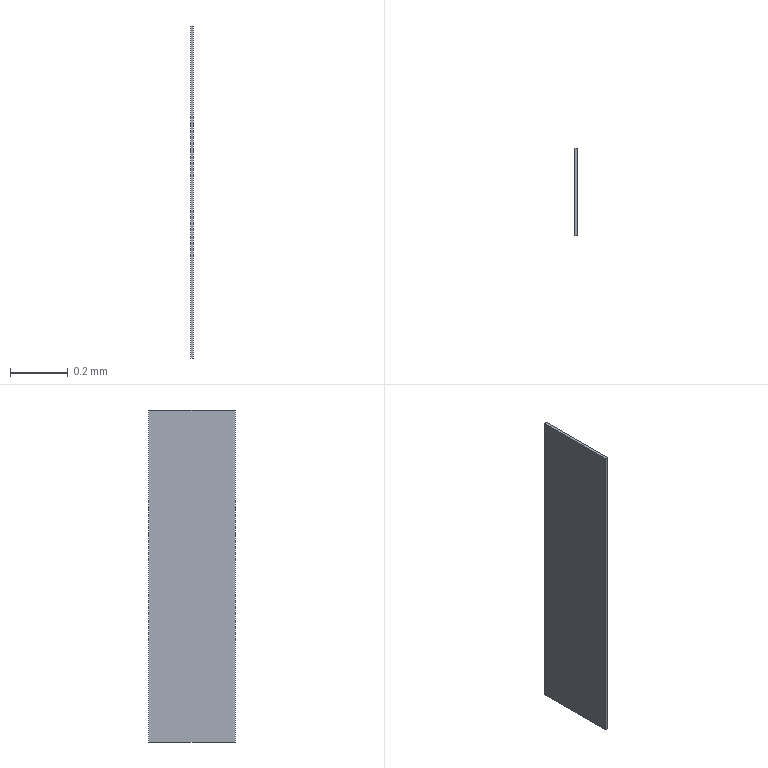Part | Creo | 1 solid | 6 faces | box 0.01 x 0.3 x 1.15 mm | volume 0.00345 mm3 | plane 6
STEP:
#1=CARTESIAN_POINT('',(0.,0.,0.));
#2=DIRECTION('',(0.,0.,1.));
#3=DIRECTION('',(1.,0.,0.));
#4=AXIS2_PLACEMENT_3D('',#1,#2,#3);
#5=CARTESIAN_POINT('',(0.12,-6.2,0.525));
#6=VERTEX_POINT('',#5);
#7=CARTESIAN_POINT('',(0.12,-6.2,1.675));
#8=VERTEX_POINT('',#7);
#9=CARTESIAN_POINT('',(0.12,-6.2,0.525));
#10=DIRECTION('',(0.,0.,1.));
#11=VECTOR('',#10,1.15);
#12=LINE('',#9,#11);
#13=EDGE_CURVE('',#6,#8,#12,.T.);
#14=ORIENTED_EDGE('',*,*,#13,.F.);
#15=CARTESIAN_POINT('',(0.12,-6.5,0.525));
#16=VERTEX_POINT('',#15);
#17=CARTESIAN_POINT('',(0.12,-6.5,0.525));
#18=DIRECTION('',(0.,1.,0.));
#19=VECTOR('',#18,0.3);
#20=LINE('',#17,#19);
#21=EDGE_CURVE('',#16,#6,#20,.T.);
#22=ORIENTED_EDGE('',*,*,#21,.F.);
#23=CARTESIAN_POINT('',(0.12,-6.5,1.675));
#24=VERTEX_POINT('',#23);
#25=CARTESIAN_POINT('',(0.12,-6.5,1.675));
#26=DIRECTION('',(0.,0.,-1.));
#27=VECTOR('',#26,1.15);
#28=LINE('',#25,#27);
#29=EDGE_CURVE('',#24,#16,#28,.T.);
#30=ORIENTED_EDGE('',*,*,#29,.F.);
#31=CARTESIAN_POINT('',(0.12,-6.2,1.675));
#32=DIRECTION('',(0.,-1.,0.));
#33=VECTOR('',#32,0.3);
#34=LINE('',#31,#33);
#35=EDGE_CURVE('',#8,#24,#34,.T.);
#36=ORIENTED_EDGE('',*,*,#35,.F.);
#37=EDGE_LOOP('',(#14,#22,#30,#36));
#38=FACE_OUTER_BOUND('',#37,.F.);
#39=CARTESIAN_POINT('',(0.12,0.,0.));
#40=DIRECTION('',(1.,0.,0.));
#41=DIRECTION('',(0.,-1.,0.));
#42=AXIS2_PLACEMENT_3D('',#39,#40,#41);
#43=PLANE('',#42);
#44=ADVANCED_FACE('',(#38),#43,.T.);
#45=CARTESIAN_POINT('',(0.11,-6.2,0.525));
#46=VERTEX_POINT('',#45);
#47=CARTESIAN_POINT('',(0.11,-6.2,1.675));
#48=VERTEX_POINT('',#47);
#49=CARTESIAN_POINT('',(0.11,-6.2,0.525));
#50=DIRECTION('',(0.,0.,1.));
#51=VECTOR('',#50,1.15);
#52=LINE('',#49,#51);
#53=EDGE_CURVE('',#46,#48,#52,.T.);
#54=ORIENTED_EDGE('',*,*,#53,.F.);
#55=CARTESIAN_POINT('',(0.11,-6.2,0.525));
#56=DIRECTION('',(1.,0.,0.));
#57=VECTOR('',#56,0.01);
#58=LINE('',#55,#57);
#59=EDGE_CURVE('',#46,#6,#58,.T.);
#60=ORIENTED_EDGE('',*,*,#59,.T.);
#61=ORIENTED_EDGE('',*,*,#13,.T.);
#62=CARTESIAN_POINT('',(0.11,-6.2,1.675));
#63=DIRECTION('',(1.,0.,0.));
#64=VECTOR('',#63,0.01);
#65=LINE('',#62,#64);
#66=EDGE_CURVE('',#48,#8,#65,.T.);
#67=ORIENTED_EDGE('',*,*,#66,.F.);
#68=EDGE_LOOP('',(#54,#60,#61,#67));
#69=FACE_OUTER_BOUND('',#68,.F.);
#70=CARTESIAN_POINT('',(0.,-6.2,0.525));
#71=DIRECTION('',(0.,1.,0.));
#72=DIRECTION('',(0.,0.,1.));
#73=AXIS2_PLACEMENT_3D('',#70,#71,#72);
#74=PLANE('',#73);
#75=ADVANCED_FACE('',(#69),#74,.T.);
#76=ORIENTED_EDGE('',*,*,#53,.T.);
#77=CARTESIAN_POINT('',(0.11,-6.5,1.675));
#78=VERTEX_POINT('',#77);
#79=CARTESIAN_POINT('',(0.11,-6.2,1.675));
#80=DIRECTION('',(0.,-1.,0.));
#81=VECTOR('',#80,0.3);
#82=LINE('',#79,#81);
#83=EDGE_CURVE('',#48,#78,#82,.T.);
#84=ORIENTED_EDGE('',*,*,#83,.T.);
#85=CARTESIAN_POINT('',(0.11,-6.5,0.525));
#86=VERTEX_POINT('',#85);
#87=CARTESIAN_POINT('',(0.11,-6.5,1.675));
#88=DIRECTION('',(0.,0.,-1.));
#89=VECTOR('',#88,1.15);
#90=LINE('',#87,#89);
#91=EDGE_CURVE('',#78,#86,#90,.T.);
#92=ORIENTED_EDGE('',*,*,#91,.T.);
#93=CARTESIAN_POINT('',(0.11,-6.5,0.525));
#94=DIRECTION('',(0.,1.,0.));
#95=VECTOR('',#94,0.3);
#96=LINE('',#93,#95);
#97=EDGE_CURVE('',#86,#46,#96,.T.);
#98=ORIENTED_EDGE('',*,*,#97,.T.);
#99=EDGE_LOOP('',(#76,#84,#92,#98));
#100=FACE_OUTER_BOUND('',#99,.F.);
#101=CARTESIAN_POINT('',(0.11,-11.395,4.186));
#102=DIRECTION('',(1.,0.,0.));
#103=DIRECTION('',(0.,1.,0.));
#104=AXIS2_PLACEMENT_3D('',#101,#102,#103);
#105=PLANE('',#104);
#106=ADVANCED_FACE('',(#100),#105,.F.);
#107=ORIENTED_EDGE('',*,*,#83,.F.);
#108=ORIENTED_EDGE('',*,*,#66,.T.);
#109=ORIENTED_EDGE('',*,*,#35,.T.);
#110=CARTESIAN_POINT('',(0.11,-6.5,1.675));
#111=DIRECTION('',(1.,0.,0.));
#112=VECTOR('',#111,0.01);
#113=LINE('',#110,#112);
#114=EDGE_CURVE('',#78,#24,#113,.T.);
#115=ORIENTED_EDGE('',*,*,#114,.F.);
#116=EDGE_LOOP('',(#107,#108,#109,#115));
#117=FACE_OUTER_BOUND('',#116,.F.);
#118=CARTESIAN_POINT('',(0.,-6.2,1.675));
#119=DIRECTION('',(0.,0.,1.));
#120=DIRECTION('',(0.,-1.,0.));
#121=AXIS2_PLACEMENT_3D('',#118,#119,#120);
#122=PLANE('',#121);
#123=ADVANCED_FACE('',(#117),#122,.T.);
#124=ORIENTED_EDGE('',*,*,#91,.F.);
#125=ORIENTED_EDGE('',*,*,#114,.T.);
#126=ORIENTED_EDGE('',*,*,#29,.T.);
#127=CARTESIAN_POINT('',(0.11,-6.5,0.525));
#128=DIRECTION('',(1.,0.,0.));
#129=VECTOR('',#128,0.01);
#130=LINE('',#127,#129);
#131=EDGE_CURVE('',#86,#16,#130,.T.);
#132=ORIENTED_EDGE('',*,*,#131,.F.);
#133=EDGE_LOOP('',(#124,#125,#126,#132));
#134=FACE_OUTER_BOUND('',#133,.F.);
#135=CARTESIAN_POINT('',(0.,-6.5,1.675));
#136=DIRECTION('',(0.,-1.,0.));
#137=DIRECTION('',(0.,0.,-1.));
#138=AXIS2_PLACEMENT_3D('',#135,#136,#137);
#139=PLANE('',#138);
#140=ADVANCED_FACE('',(#134),#139,.T.);
#141=ORIENTED_EDGE('',*,*,#97,.F.);
#142=ORIENTED_EDGE('',*,*,#131,.T.);
#143=ORIENTED_EDGE('',*,*,#21,.T.);
#144=ORIENTED_EDGE('',*,*,#59,.F.);
#145=EDGE_LOOP('',(#141,#142,#143,#144));
#146=FACE_OUTER_BOUND('',#145,.F.);
#147=CARTESIAN_POINT('',(0.,-6.5,0.525));
#148=DIRECTION('',(0.,0.,-1.));
#149=DIRECTION('',(0.,1.,0.));
#150=AXIS2_PLACEMENT_3D('',#147,#148,#149);
#151=PLANE('',#150);
#152=ADVANCED_FACE('',(#146),#151,.T.);
#153=CLOSED_SHELL('',(#44,#75,#106,#123,#140,#152));
#154=MANIFOLD_SOLID_BREP('',#153);
#155=(LENGTH_UNIT()NAMED_UNIT(*)SI_UNIT(.MILLI.,.METRE.));
#156=UNCERTAINTY_MEASURE_WITH_UNIT(LENGTH_MEASURE(0.0001188),#155,'','');
#157=(NAMED_UNIT(*)PLANE_ANGLE_UNIT()SI_UNIT($,.RADIAN.));
#158=PLANE_ANGLE_MEASURE_WITH_UNIT(PLANE_ANGLE_MEASURE(0.01745),#157);
#159=(CONVERSION_BASED_UNIT('DEGREE',#158)NAMED_UNIT(*)PLANE_ANGLE_UNIT());
#160=(NAMED_UNIT(*)SI_UNIT($,.STERADIAN.)SOLID_ANGLE_UNIT());
#161=(GEOMETRIC_REPRESENTATION_CONTEXT(3)GLOBAL_UNCERTAINTY_ASSIGNED_CONTEXT((#156))GLOBAL_UNIT_ASSIGNED_CONTEXT((#155,#159,#160))REPRESENTATION_CONTEXT('',''));
#162=ADVANCED_BREP_SHAPE_REPRESENTATION('',(#4,#154),#161);